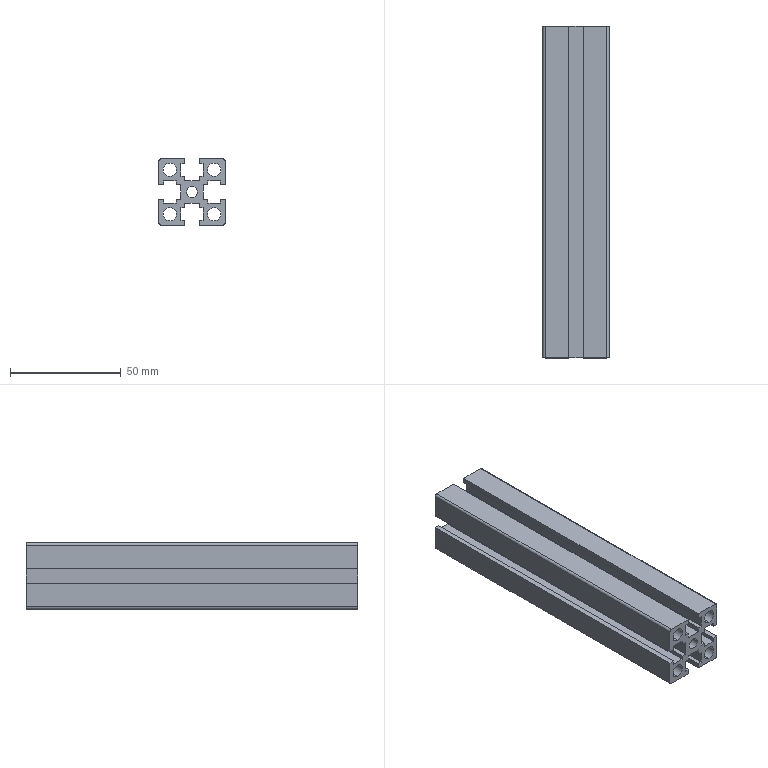Part | STEP file | 02-16 Belt line support foot | 1 solid | 76 faces | box 30 x 150 x 30 mm | volume 64799 mm3 | plane 54 | cylinder 18 | cone 4 | commonest cylinder face diameters 6 x8 2 x4 5 x4 4.9 x2